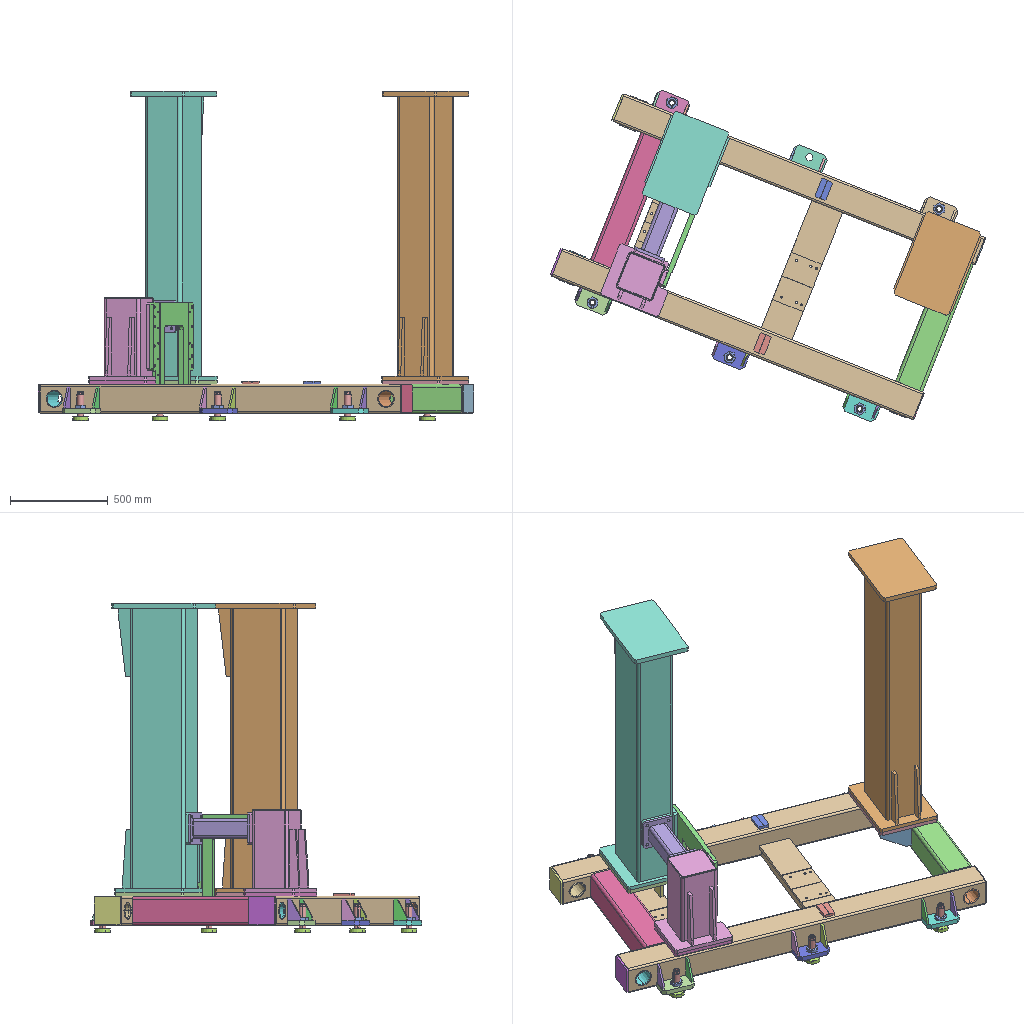Assembly | SolidWorks | 9 different items | 21 placed | box 2225 x 1693 x 1683 mm
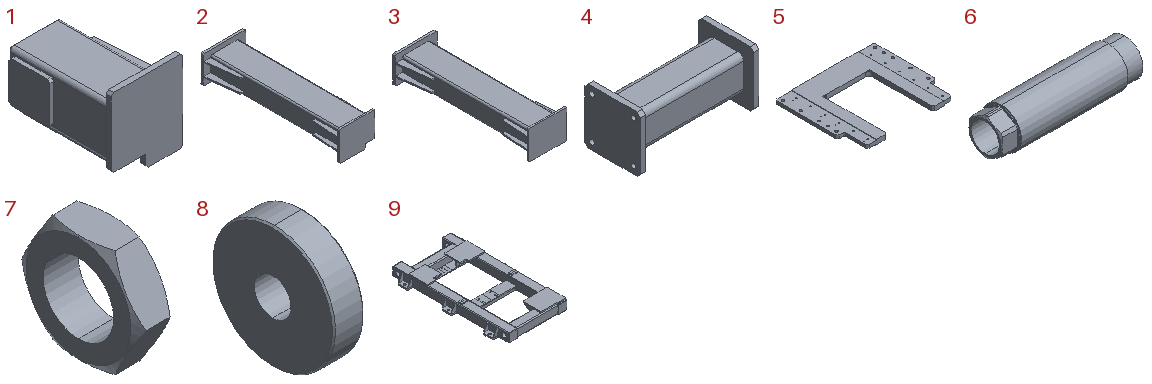Parts list (item | quantity | size | volume | features):
1 | x1 | 280 x 420 x 320 mm | 5533636 mm3 | features ICE 5, Chamfer 2, Extrusion 1, Fillet 1, MirrorPattern 1
2 | x1 | 460 x 1476 x 320 mm | 18498922 mm3 | features ICE 6, MirrorPattern 2, Extrusion 1
3 | x1 | 460 x 1476 x 320 mm | 20749959 mm3 | features ICE 4, MirrorPattern 2, Extrusion 1
4 | x1 | 340 x 160 x 160 mm | 1614311 mm3 | features 3DProfileFeature 1, Extrusion 1, HoleWzd 1, ICE 1, MirrorPattern 1
5 | x1 | 556 x 480 x 25 mm | 3535416 mm3 | features 3DProfileFeature 5, HoleWzd 5, ICE 3, MirrorPattern 2, Chamfer 1, Extrusion 1, Fillet 1
6 | x5 | 129.156 x 36 x 36 mm | 58717 mm3 | features Cut 4, RevCut 2, Extrusion 1, Fillet 1
7 | x5 | 18 x 63.509 x 55 mm | 28207 mm3 | features 3DProfileFeature 1, Extrusion 1, HoleWzd 1, MirrorPattern 1, RevCut 1
8 | x5 | 20 x 80 x 80 mm | 90475 mm3 | features Chamfer 2, Cut 1, Extrusion 1
9 | x1 | 1180 x 2000 x 170 mm | 41787721 mm3 | features ICE 9, Boss 8, Chamfer 6, HoleWzd 5, LPattern 5, EndCap 4, Cut 2, MirrorSolid 1, WeldMemberFeat 1, WeldmentFeature 1
Mates (type | each side: item.copy, entity, surface, feature):
Coincident | 1.1 face plane Boss-Extrude5 | 4.1 face plane Mirror1 | 2 times
Coincident | 1.1 face plane Boss-Extrude8 | 5.1 face plane Boss-Extrude1 | 3 times
Coincident | 1.1 face plane Boss-Extrude1 | 3.1 face plane Boss-Extrude1
Coincident | 2.1 face plane Boss-Extrude2 | 3.1 face plane Boss-Extrude2 | 2 times
Coincident | 2.1 face plane Boss-Extrude5 | 4.1 face plane Boss-Extrude1 | 2 times
Coincident | 2.1 face plane Boss-Extrude10 | 5.1 face plane Boss-Extrude1 | 2 times
DistanceDim | 3.1 face plane Boss-Extrude2 | 2.1 face plane Boss-Extrude2
Coincident | 1.1 face plane Boss-Extrude1 | 9.1 face plane Extrude3
Coincident | 2.1 face plane Boss-Extrude1 | 9.1 face plane Extrude3 | 2 times
Concentric | 6.1 face cylinder Extrude1 | 8.1 face cylinder Cut-Extrude1
Concentric | 6.1 face cylinder Cut-Extrude3 | 7.1 face cylinder M36x2.0 Tapped Hole1
Perpendicular | 6.1 face plane Cut-Extrude4 | 7.1 face plane Extrude1
DistanceDim | 7.1 face plane Extrude1 | 8.1 face plane Extrude1
Concentric | 6.1 face cylinder Extrude1 | 9.1 face cylinder Extrude5
Coincident | 7.1 face plane Extrude1 | 9.1 face plane Extrude5
Tangent | 6.2 face sphere Cut-Revolve1 | 8.2 face cone Chamfer2
Concentric | 6.2 face cylinder Cut-Extrude3 | 7.2 face cylinder M36x2.0 Tapped Hole1
Perpendicular | 6.2 face plane Cut-Extrude4 | 7.2 face plane Extrude1
DistanceDim | 7.2 face plane Extrude1 | 8.2 face plane Extrude1
Concentric | 6.2 face cylinder Extrude1 | 9.1 face cylinder M36x2.0 Tapped Hole1
Coincident | 7.2 face plane Extrude1 | 9.1 face plane Extrude5
Concentric | 6.3 face cylinder Extrude1 | 8.3 face cylinder Cut-Extrude1
Tangent | 6.3 face sphere Cut-Revolve1 | 8.3 face cone Chamfer2
Concentric | 6.3 face cylinder Cut-Extrude3 | 7.3 face cylinder M36x2.0 Tapped Hole1
Perpendicular | 6.3 face plane Cut-Extrude4 | 7.3 face plane Extrude1
Concentric | 6.3 face cylinder Extrude1 | 9.1 face cylinder Extrude5
Coincident | 7.3 face plane Extrude1 | 9.1 face plane Extrude5
Concentric | 6.4 face cylinder Extrude1 | 8.4 face cylinder Cut-Extrude1
Tangent | 6.4 face sphere Cut-Revolve1 | 8.4 face cone Chamfer2
Concentric | 6.4 face cylinder Cut-Extrude3 | 7.4 face cylinder M36x2.0 Tapped Hole1
Perpendicular | 6.4 face plane Cut-Extrude4 | 7.4 face plane Extrude1
Concentric | 6.4 face cylinder Extrude1 | 9.1 face cylinder M36x2.0 Tapped Hole1
Coincident | 7.4 face plane Extrude1 | 9.1 face plane Extrude5
Concentric | 6.5 face cylinder Extrude1 | 8.5 face cylinder Cut-Extrude1
Tangent | 6.5 face sphere Cut-Revolve1 | 8.5 face cone Chamfer2
Concentric | 6.5 face cylinder Cut-Extrude3 | 7.5 face cylinder M36x2.0 Tapped Hole1
Perpendicular | 6.5 face plane Cut-Extrude4 | 7.5 face plane Extrude1
DistanceDim | 7.5 face plane Extrude1 | 8.5 face plane Extrude1
Concentric | 6.5 face cylinder Extrude1 | 9.1 face cylinder M36x2.0 Tapped Hole1